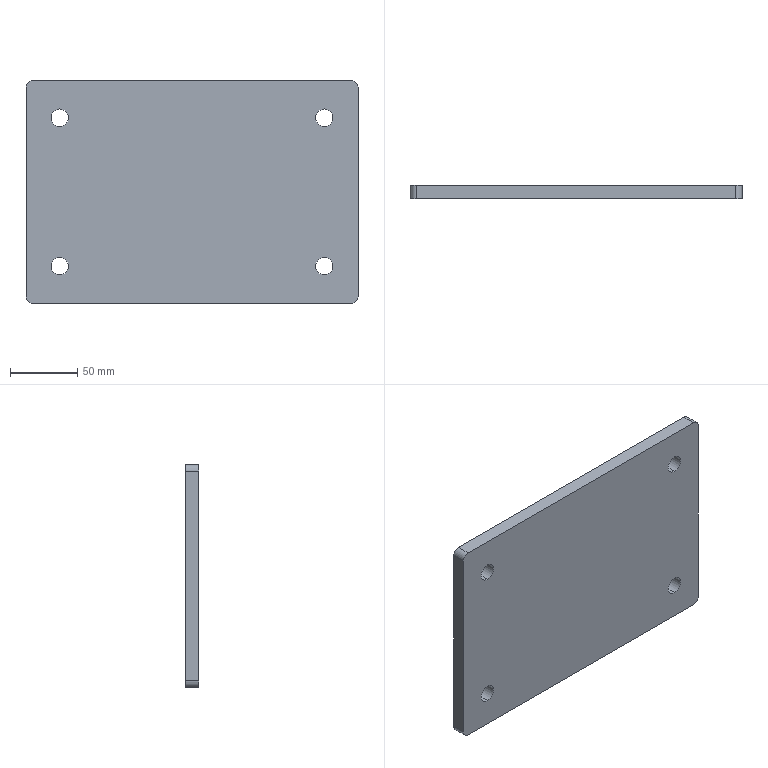Part | SolidWorks | features BaseBody 1 | 1 solid | 18 faces | box 246 x 10 x 165 mm | volume 400376 mm3 | cylinder 12 | plane 6 | commonest cylinder face diameters 13 x8 10 x4
STEP:
#1=CARTESIAN_POINT('',(-98.,0.,61.5));
#2=VERTEX_POINT('',#1);
#3=CARTESIAN_POINT('',(-98.,0.,48.5));
#4=VERTEX_POINT('',#3);
#5=CARTESIAN_POINT('',(-98.,0.,55.));
#6=DIRECTION('',(0.,-1.,0.));
#7=DIRECTION('',(0.,0.,1.));
#8=AXIS2_PLACEMENT_3D('',#5,#6,#7);
#9=CIRCLE('',#8,6.5);
#10=EDGE_CURVE('',#2,#4,#9,.T.);
#11=ORIENTED_EDGE('',*,*,#10,.T.);
#12=CARTESIAN_POINT('',(-98.,10.,48.5));
#13=VERTEX_POINT('',#12);
#14=CARTESIAN_POINT('',(-98.,-286.38,48.5));
#15=DIRECTION('',(0.,1.,0.));
#16=VECTOR('',#15,1000.);
#17=LINE('',#14,#16);
#18=EDGE_CURVE('',#4,#13,#17,.T.);
#19=ORIENTED_EDGE('',*,*,#18,.T.);
#20=CARTESIAN_POINT('',(-98.,10.,61.5));
#21=VERTEX_POINT('',#20);
#22=CARTESIAN_POINT('',(-98.,10.,55.));
#23=DIRECTION('',(0.,-1.,0.));
#24=DIRECTION('',(0.,0.,1.));
#25=AXIS2_PLACEMENT_3D('',#22,#23,#24);
#26=CIRCLE('',#25,6.5);
#27=EDGE_CURVE('',#21,#13,#26,.T.);
#28=ORIENTED_EDGE('',*,*,#27,.F.);
#29=CARTESIAN_POINT('',(-98.,-286.38,61.5));
#30=DIRECTION('',(0.,1.,0.));
#31=VECTOR('',#30,1000.);
#32=LINE('',#29,#31);
#33=EDGE_CURVE('',#2,#21,#32,.T.);
#34=ORIENTED_EDGE('',*,*,#33,.F.);
#35=EDGE_LOOP('',(#11,#19,#28,#34));
#36=FACE_OUTER_BOUND('',#35,.T.);
#37=CARTESIAN_POINT('',(-98.,-286.38,55.));
#38=DIRECTION('',(0.,1.,0.));
#39=DIRECTION('',(0.,0.,1.));
#40=AXIS2_PLACEMENT_3D('',#37,#38,#39);
#41=CYLINDRICAL_SURFACE('',#40,6.5);
#42=ADVANCED_FACE('',(#36),#41,.F.);
#43=CARTESIAN_POINT('',(-98.,0.,-48.5));
#44=VERTEX_POINT('',#43);
#45=CARTESIAN_POINT('',(-98.,0.,-61.5));
#46=VERTEX_POINT('',#45);
#47=CARTESIAN_POINT('',(-98.,0.,-55.));
#48=DIRECTION('',(0.,-1.,0.));
#49=DIRECTION('',(0.,0.,1.));
#50=AXIS2_PLACEMENT_3D('',#47,#48,#49);
#51=CIRCLE('',#50,6.5);
#52=EDGE_CURVE('',#44,#46,#51,.T.);
#53=ORIENTED_EDGE('',*,*,#52,.T.);
#54=CARTESIAN_POINT('',(-98.,10.,-61.5));
#55=VERTEX_POINT('',#54);
#56=CARTESIAN_POINT('',(-98.,-286.38,-61.5));
#57=DIRECTION('',(0.,1.,0.));
#58=VECTOR('',#57,1000.);
#59=LINE('',#56,#58);
#60=EDGE_CURVE('',#46,#55,#59,.T.);
#61=ORIENTED_EDGE('',*,*,#60,.T.);
#62=CARTESIAN_POINT('',(-98.,10.,-48.5));
#63=VERTEX_POINT('',#62);
#64=CARTESIAN_POINT('',(-98.,10.,-55.));
#65=DIRECTION('',(0.,-1.,0.));
#66=DIRECTION('',(0.,0.,1.));
#67=AXIS2_PLACEMENT_3D('',#64,#65,#66);
#68=CIRCLE('',#67,6.5);
#69=EDGE_CURVE('',#63,#55,#68,.T.);
#70=ORIENTED_EDGE('',*,*,#69,.F.);
#71=CARTESIAN_POINT('',(-98.,-286.38,-48.5));
#72=DIRECTION('',(0.,1.,0.));
#73=VECTOR('',#72,1000.);
#74=LINE('',#71,#73);
#75=EDGE_CURVE('',#44,#63,#74,.T.);
#76=ORIENTED_EDGE('',*,*,#75,.F.);
#77=EDGE_LOOP('',(#53,#61,#70,#76));
#78=FACE_OUTER_BOUND('',#77,.T.);
#79=CARTESIAN_POINT('',(-98.,-286.38,-55.));
#80=DIRECTION('',(0.,1.,0.));
#81=DIRECTION('',(0.,0.,1.));
#82=AXIS2_PLACEMENT_3D('',#79,#80,#81);
#83=CYLINDRICAL_SURFACE('',#82,6.5);
#84=ADVANCED_FACE('',(#78),#83,.F.);
#85=CARTESIAN_POINT('',(98.,0.,61.5));
#86=VERTEX_POINT('',#85);
#87=CARTESIAN_POINT('',(98.,0.,48.5));
#88=VERTEX_POINT('',#87);
#89=CARTESIAN_POINT('',(98.,0.,55.));
#90=DIRECTION('',(0.,-1.,0.));
#91=DIRECTION('',(0.,0.,1.));
#92=AXIS2_PLACEMENT_3D('',#89,#90,#91);
#93=CIRCLE('',#92,6.5);
#94=EDGE_CURVE('',#86,#88,#93,.T.);
#95=ORIENTED_EDGE('',*,*,#94,.T.);
#96=CARTESIAN_POINT('',(98.,10.,48.5));
#97=VERTEX_POINT('',#96);
#98=CARTESIAN_POINT('',(98.,-286.38,48.5));
#99=DIRECTION('',(0.,1.,0.));
#100=VECTOR('',#99,1000.);
#101=LINE('',#98,#100);
#102=EDGE_CURVE('',#88,#97,#101,.T.);
#103=ORIENTED_EDGE('',*,*,#102,.T.);
#104=CARTESIAN_POINT('',(98.,10.,61.5));
#105=VERTEX_POINT('',#104);
#106=CARTESIAN_POINT('',(98.,10.,55.));
#107=DIRECTION('',(0.,-1.,0.));
#108=DIRECTION('',(0.,0.,1.));
#109=AXIS2_PLACEMENT_3D('',#106,#107,#108);
#110=CIRCLE('',#109,6.5);
#111=EDGE_CURVE('',#105,#97,#110,.T.);
#112=ORIENTED_EDGE('',*,*,#111,.F.);
#113=CARTESIAN_POINT('',(98.,-286.38,61.5));
#114=DIRECTION('',(0.,1.,0.));
#115=VECTOR('',#114,1000.);
#116=LINE('',#113,#115);
#117=EDGE_CURVE('',#86,#105,#116,.T.);
#118=ORIENTED_EDGE('',*,*,#117,.F.);
#119=EDGE_LOOP('',(#95,#103,#112,#118));
#120=FACE_OUTER_BOUND('',#119,.T.);
#121=CARTESIAN_POINT('',(98.,-286.38,55.));
#122=DIRECTION('',(0.,1.,0.));
#123=DIRECTION('',(0.,0.,1.));
#124=AXIS2_PLACEMENT_3D('',#121,#122,#123);
#125=CYLINDRICAL_SURFACE('',#124,6.5);
#126=ADVANCED_FACE('',(#120),#125,.F.);
#127=CARTESIAN_POINT('',(98.,0.,-48.5));
#128=VERTEX_POINT('',#127);
#129=CARTESIAN_POINT('',(98.,0.,-61.5));
#130=VERTEX_POINT('',#129);
#131=CARTESIAN_POINT('',(98.,0.,-55.));
#132=DIRECTION('',(0.,-1.,0.));
#133=DIRECTION('',(0.,0.,1.));
#134=AXIS2_PLACEMENT_3D('',#131,#132,#133);
#135=CIRCLE('',#134,6.5);
#136=EDGE_CURVE('',#128,#130,#135,.T.);
#137=ORIENTED_EDGE('',*,*,#136,.T.);
#138=CARTESIAN_POINT('',(98.,10.,-61.5));
#139=VERTEX_POINT('',#138);
#140=CARTESIAN_POINT('',(98.,-286.38,-61.5));
#141=DIRECTION('',(0.,1.,0.));
#142=VECTOR('',#141,1000.);
#143=LINE('',#140,#142);
#144=EDGE_CURVE('',#130,#139,#143,.T.);
#145=ORIENTED_EDGE('',*,*,#144,.T.);
#146=CARTESIAN_POINT('',(98.,10.,-48.5));
#147=VERTEX_POINT('',#146);
#148=CARTESIAN_POINT('',(98.,10.,-55.));
#149=DIRECTION('',(0.,-1.,0.));
#150=DIRECTION('',(0.,0.,1.));
#151=AXIS2_PLACEMENT_3D('',#148,#149,#150);
#152=CIRCLE('',#151,6.5);
#153=EDGE_CURVE('',#147,#139,#152,.T.);
#154=ORIENTED_EDGE('',*,*,#153,.F.);
#155=CARTESIAN_POINT('',(98.,-286.38,-48.5));
#156=DIRECTION('',(0.,1.,0.));
#157=VECTOR('',#156,1000.);
#158=LINE('',#155,#157);
#159=EDGE_CURVE('',#128,#147,#158,.T.);
#160=ORIENTED_EDGE('',*,*,#159,.F.);
#161=EDGE_LOOP('',(#137,#145,#154,#160));
#162=FACE_OUTER_BOUND('',#161,.T.);
#163=CARTESIAN_POINT('',(98.,-286.38,-55.));
#164=DIRECTION('',(0.,1.,0.));
#165=DIRECTION('',(0.,0.,1.));
#166=AXIS2_PLACEMENT_3D('',#163,#164,#165);
#167=CYLINDRICAL_SURFACE('',#166,6.5);
#168=ADVANCED_FACE('',(#162),#167,.F.);
#169=ORIENTED_EDGE('',*,*,#10,.F.);
#170=CARTESIAN_POINT('',(-98.,0.,55.));
#171=DIRECTION('',(0.,-1.,0.));
#172=DIRECTION('',(0.,0.,1.));
#173=AXIS2_PLACEMENT_3D('',#170,#171,#172);
#174=CIRCLE('',#173,6.5);
#175=EDGE_CURVE('',#4,#2,#174,.T.);
#176=ORIENTED_EDGE('',*,*,#175,.F.);
#177=EDGE_LOOP('',(#169,#176));
#178=FACE_BOUND('',#177,.T.);
#179=ORIENTED_EDGE('',*,*,#52,.F.);
#180=CARTESIAN_POINT('',(-98.,0.,-55.));
#181=DIRECTION('',(0.,-1.,0.));
#182=DIRECTION('',(0.,0.,1.));
#183=AXIS2_PLACEMENT_3D('',#180,#181,#182);
#184=CIRCLE('',#183,6.5);
#185=EDGE_CURVE('',#46,#44,#184,.T.);
#186=ORIENTED_EDGE('',*,*,#185,.F.);
#187=EDGE_LOOP('',(#179,#186));
#188=FACE_BOUND('',#187,.T.);
#189=ORIENTED_EDGE('',*,*,#94,.F.);
#190=CARTESIAN_POINT('',(98.,0.,55.));
#191=DIRECTION('',(0.,-1.,0.));
#192=DIRECTION('',(0.,0.,1.));
#193=AXIS2_PLACEMENT_3D('',#190,#191,#192);
#194=CIRCLE('',#193,6.5);
#195=EDGE_CURVE('',#88,#86,#194,.T.);
#196=ORIENTED_EDGE('',*,*,#195,.F.);
#197=EDGE_LOOP('',(#189,#196));
#198=FACE_BOUND('',#197,.T.);
#199=ORIENTED_EDGE('',*,*,#136,.F.);
#200=CARTESIAN_POINT('',(98.,0.,-55.));
#201=DIRECTION('',(0.,-1.,0.));
#202=DIRECTION('',(0.,0.,1.));
#203=AXIS2_PLACEMENT_3D('',#200,#201,#202);
#204=CIRCLE('',#203,6.5);
#205=EDGE_CURVE('',#130,#128,#204,.T.);
#206=ORIENTED_EDGE('',*,*,#205,.F.);
#207=EDGE_LOOP('',(#199,#206));
#208=FACE_BOUND('',#207,.T.);
#209=CARTESIAN_POINT('',(118.,0.,-82.5));
#210=VERTEX_POINT('',#209);
#211=CARTESIAN_POINT('',(-118.,0.,-82.5));
#212=VERTEX_POINT('',#211);
#213=CARTESIAN_POINT('',(0.,0.,-82.5));
#214=DIRECTION('',(-1.,0.,0.));
#215=VECTOR('',#214,1000.);
#216=LINE('',#213,#215);
#217=EDGE_CURVE('',#210,#212,#216,.T.);
#218=ORIENTED_EDGE('',*,*,#217,.F.);
#219=CARTESIAN_POINT('',(123.,0.,-77.5));
#220=VERTEX_POINT('',#219);
#221=CARTESIAN_POINT('',(118.,0.,-77.5));
#222=DIRECTION('',(0.,1.,0.));
#223=DIRECTION('',(0.,0.,1.));
#224=AXIS2_PLACEMENT_3D('',#221,#222,#223);
#225=CIRCLE('',#224,5.);
#226=EDGE_CURVE('',#220,#210,#225,.T.);
#227=ORIENTED_EDGE('',*,*,#226,.F.);
#228=CARTESIAN_POINT('',(123.,0.,77.5));
#229=VERTEX_POINT('',#228);
#230=CARTESIAN_POINT('',(123.,0.,0.));
#231=DIRECTION('',(0.,0.,-1.));
#232=VECTOR('',#231,1000.);
#233=LINE('',#230,#232);
#234=EDGE_CURVE('',#229,#220,#233,.T.);
#235=ORIENTED_EDGE('',*,*,#234,.F.);
#236=CARTESIAN_POINT('',(118.,0.,82.5));
#237=VERTEX_POINT('',#236);
#238=CARTESIAN_POINT('',(118.,0.,77.5));
#239=DIRECTION('',(0.,1.,0.));
#240=DIRECTION('',(0.,0.,1.));
#241=AXIS2_PLACEMENT_3D('',#238,#239,#240);
#242=CIRCLE('',#241,5.);
#243=EDGE_CURVE('',#237,#229,#242,.T.);
#244=ORIENTED_EDGE('',*,*,#243,.F.);
#245=CARTESIAN_POINT('',(-118.,0.,82.5));
#246=VERTEX_POINT('',#245);
#247=CARTESIAN_POINT('',(0.,0.,82.5));
#248=DIRECTION('',(1.,0.,0.));
#249=VECTOR('',#248,1000.);
#250=LINE('',#247,#249);
#251=EDGE_CURVE('',#246,#237,#250,.T.);
#252=ORIENTED_EDGE('',*,*,#251,.F.);
#253=CARTESIAN_POINT('',(-123.,0.,77.5));
#254=VERTEX_POINT('',#253);
#255=CARTESIAN_POINT('',(-118.,0.,77.5));
#256=DIRECTION('',(0.,1.,0.));
#257=DIRECTION('',(0.,0.,1.));
#258=AXIS2_PLACEMENT_3D('',#255,#256,#257);
#259=CIRCLE('',#258,5.);
#260=EDGE_CURVE('',#254,#246,#259,.T.);
#261=ORIENTED_EDGE('',*,*,#260,.F.);
#262=CARTESIAN_POINT('',(-123.,0.,-77.5));
#263=VERTEX_POINT('',#262);
#264=CARTESIAN_POINT('',(-123.,0.,0.));
#265=DIRECTION('',(0.,0.,1.));
#266=VECTOR('',#265,1000.);
#267=LINE('',#264,#266);
#268=EDGE_CURVE('',#263,#254,#267,.T.);
#269=ORIENTED_EDGE('',*,*,#268,.F.);
#270=CARTESIAN_POINT('',(-118.,0.,-77.5));
#271=DIRECTION('',(0.,1.,0.));
#272=DIRECTION('',(0.,0.,1.));
#273=AXIS2_PLACEMENT_3D('',#270,#271,#272);
#274=CIRCLE('',#273,5.);
#275=EDGE_CURVE('',#212,#263,#274,.T.);
#276=ORIENTED_EDGE('',*,*,#275,.F.);
#277=EDGE_LOOP('',(#218,#227,#235,#244,#252,#261,#269,#276));
#278=FACE_OUTER_BOUND('',#277,.T.);
#279=CARTESIAN_POINT('',(0.,0.,0.));
#280=DIRECTION('',(0.,1.,0.));
#281=DIRECTION('',(0.,0.,1.));
#282=AXIS2_PLACEMENT_3D('',#279,#280,#281);
#283=PLANE('',#282);
#284=ADVANCED_FACE('',(#178,#188,#198,#208,#278),#283,.F.);
#285=ORIENTED_EDGE('',*,*,#18,.F.);
#286=ORIENTED_EDGE('',*,*,#175,.T.);
#287=ORIENTED_EDGE('',*,*,#33,.T.);
#288=CARTESIAN_POINT('',(-98.,10.,55.));
#289=DIRECTION('',(0.,-1.,0.));
#290=DIRECTION('',(0.,0.,1.));
#291=AXIS2_PLACEMENT_3D('',#288,#289,#290);
#292=CIRCLE('',#291,6.5);
#293=EDGE_CURVE('',#13,#21,#292,.T.);
#294=ORIENTED_EDGE('',*,*,#293,.F.);
#295=EDGE_LOOP('',(#285,#286,#287,#294));
#296=FACE_OUTER_BOUND('',#295,.T.);
#297=CARTESIAN_POINT('',(-98.,-286.38,55.));
#298=DIRECTION('',(0.,1.,0.));
#299=DIRECTION('',(0.,0.,1.));
#300=AXIS2_PLACEMENT_3D('',#297,#298,#299);
#301=CYLINDRICAL_SURFACE('',#300,6.5);
#302=ADVANCED_FACE('',(#296),#301,.F.);
#303=ORIENTED_EDGE('',*,*,#60,.F.);
#304=ORIENTED_EDGE('',*,*,#185,.T.);
#305=ORIENTED_EDGE('',*,*,#75,.T.);
#306=CARTESIAN_POINT('',(-98.,10.,-55.));
#307=DIRECTION('',(0.,-1.,0.));
#308=DIRECTION('',(0.,0.,1.));
#309=AXIS2_PLACEMENT_3D('',#306,#307,#308);
#310=CIRCLE('',#309,6.5);
#311=EDGE_CURVE('',#55,#63,#310,.T.);
#312=ORIENTED_EDGE('',*,*,#311,.F.);
#313=EDGE_LOOP('',(#303,#304,#305,#312));
#314=FACE_OUTER_BOUND('',#313,.T.);
#315=CARTESIAN_POINT('',(-98.,-286.38,-55.));
#316=DIRECTION('',(0.,1.,0.));
#317=DIRECTION('',(0.,0.,1.));
#318=AXIS2_PLACEMENT_3D('',#315,#316,#317);
#319=CYLINDRICAL_SURFACE('',#318,6.5);
#320=ADVANCED_FACE('',(#314),#319,.F.);
#321=ORIENTED_EDGE('',*,*,#102,.F.);
#322=ORIENTED_EDGE('',*,*,#195,.T.);
#323=ORIENTED_EDGE('',*,*,#117,.T.);
#324=CARTESIAN_POINT('',(98.,10.,55.));
#325=DIRECTION('',(0.,-1.,0.));
#326=DIRECTION('',(0.,0.,1.));
#327=AXIS2_PLACEMENT_3D('',#324,#325,#326);
#328=CIRCLE('',#327,6.5);
#329=EDGE_CURVE('',#97,#105,#328,.T.);
#330=ORIENTED_EDGE('',*,*,#329,.F.);
#331=EDGE_LOOP('',(#321,#322,#323,#330));
#332=FACE_OUTER_BOUND('',#331,.T.);
#333=CARTESIAN_POINT('',(98.,-286.38,55.));
#334=DIRECTION('',(0.,1.,0.));
#335=DIRECTION('',(0.,0.,1.));
#336=AXIS2_PLACEMENT_3D('',#333,#334,#335);
#337=CYLINDRICAL_SURFACE('',#336,6.5);
#338=ADVANCED_FACE('',(#332),#337,.F.);
#339=ORIENTED_EDGE('',*,*,#144,.F.);
#340=ORIENTED_EDGE('',*,*,#205,.T.);
#341=ORIENTED_EDGE('',*,*,#159,.T.);
#342=CARTESIAN_POINT('',(98.,10.,-55.));
#343=DIRECTION('',(0.,-1.,0.));
#344=DIRECTION('',(0.,0.,1.));
#345=AXIS2_PLACEMENT_3D('',#342,#343,#344);
#346=CIRCLE('',#345,6.5);
#347=EDGE_CURVE('',#139,#147,#346,.T.);
#348=ORIENTED_EDGE('',*,*,#347,.F.);
#349=EDGE_LOOP('',(#339,#340,#341,#348));
#350=FACE_OUTER_BOUND('',#349,.T.);
#351=CARTESIAN_POINT('',(98.,-286.38,-55.));
#352=DIRECTION('',(0.,1.,0.));
#353=DIRECTION('',(0.,0.,1.));
#354=AXIS2_PLACEMENT_3D('',#351,#352,#353);
#355=CYLINDRICAL_SURFACE('',#354,6.5);
#356=ADVANCED_FACE('',(#350),#355,.F.);
#357=ORIENTED_EDGE('',*,*,#275,.T.);
#358=CARTESIAN_POINT('',(-123.,10.,-77.5));
#359=VERTEX_POINT('',#358);
#360=CARTESIAN_POINT('',(-123.,0.,-77.5));
#361=DIRECTION('',(0.,1.,0.));
#362=VECTOR('',#361,1000.);
#363=LINE('',#360,#362);
#364=EDGE_CURVE('',#263,#359,#363,.T.);
#365=ORIENTED_EDGE('',*,*,#364,.T.);
#366=CARTESIAN_POINT('',(-118.,10.,-82.5));
#367=VERTEX_POINT('',#366);
#368=CARTESIAN_POINT('',(-118.,10.,-77.5));
#369=DIRECTION('',(0.,-1.,0.));
#370=DIRECTION('',(0.,0.,1.));
#371=AXIS2_PLACEMENT_3D('',#368,#369,#370);
#372=CIRCLE('',#371,5.);
#373=EDGE_CURVE('',#359,#367,#372,.T.);
#374=ORIENTED_EDGE('',*,*,#373,.T.);
#375=CARTESIAN_POINT('',(-118.,0.,-82.5));
#376=DIRECTION('',(0.,-1.,0.));
#377=VECTOR('',#376,1000.);
#378=LINE('',#375,#377);
#379=EDGE_CURVE('',#367,#212,#378,.T.);
#380=ORIENTED_EDGE('',*,*,#379,.T.);
#381=EDGE_LOOP('',(#357,#365,#374,#380));
#382=FACE_OUTER_BOUND('',#381,.T.);
#383=CARTESIAN_POINT('',(-118.,0.,-77.5));
#384=DIRECTION('',(0.,1.,0.));
#385=DIRECTION('',(0.,0.,1.));
#386=AXIS2_PLACEMENT_3D('',#383,#384,#385);
#387=CYLINDRICAL_SURFACE('',#386,5.);
#388=ADVANCED_FACE('',(#382),#387,.T.);
#389=CARTESIAN_POINT('',(118.,10.,-82.5));
#390=VERTEX_POINT('',#389);
#391=CARTESIAN_POINT('',(118.,0.,-82.5));
#392=DIRECTION('',(0.,-1.,0.));
#393=VECTOR('',#392,1000.);
#394=LINE('',#391,#393);
#395=EDGE_CURVE('',#390,#210,#394,.T.);
#396=ORIENTED_EDGE('',*,*,#395,.T.);
#397=ORIENTED_EDGE('',*,*,#217,.T.);
#398=ORIENTED_EDGE('',*,*,#379,.F.);
#399=CARTESIAN_POINT('',(123.,10.,-82.5));
#400=DIRECTION('',(1.,0.,0.));
#401=VECTOR('',#400,1000.);
#402=LINE('',#399,#401);
#403=EDGE_CURVE('',#367,#390,#402,.T.);
#404=ORIENTED_EDGE('',*,*,#403,.T.);
#405=EDGE_LOOP('',(#396,#397,#398,#404));
#406=FACE_OUTER_BOUND('',#405,.T.);
#407=CARTESIAN_POINT('',(123.,0.,-82.5));
#408=DIRECTION('',(0.,0.,-1.));
#409=DIRECTION('',(-1.,0.,0.));
#410=AXIS2_PLACEMENT_3D('',#407,#408,#409);
#411=PLANE('',#410);
#412=ADVANCED_FACE('',(#406),#411,.T.);
#413=ORIENTED_EDGE('',*,*,#226,.T.);
#414=ORIENTED_EDGE('',*,*,#395,.F.);
#415=CARTESIAN_POINT('',(123.,10.,-77.5));
#416=VERTEX_POINT('',#415);
#417=CARTESIAN_POINT('',(118.,10.,-77.5));
#418=DIRECTION('',(0.,-1.,0.));
#419=DIRECTION('',(0.,0.,1.));
#420=AXIS2_PLACEMENT_3D('',#417,#418,#419);
#421=CIRCLE('',#420,5.);
#422=EDGE_CURVE('',#390,#416,#421,.T.);
#423=ORIENTED_EDGE('',*,*,#422,.T.);
#424=CARTESIAN_POINT('',(123.,0.,-77.5));
#425=DIRECTION('',(0.,-1.,0.));
#426=VECTOR('',#425,1000.);
#427=LINE('',#424,#426);
#428=EDGE_CURVE('',#416,#220,#427,.T.);
#429=ORIENTED_EDGE('',*,*,#428,.T.);
#430=EDGE_LOOP('',(#413,#414,#423,#429));
#431=FACE_OUTER_BOUND('',#430,.T.);
#432=CARTESIAN_POINT('',(118.,0.,-77.5));
#433=DIRECTION('',(0.,1.,0.));
#434=DIRECTION('',(0.,0.,1.));
#435=AXIS2_PLACEMENT_3D('',#432,#433,#434);
#436=CYLINDRICAL_SURFACE('',#435,5.);
#437=ADVANCED_FACE('',(#431),#436,.T.);
#438=CARTESIAN_POINT('',(123.,10.,77.5));
#439=VERTEX_POINT('',#438);
#440=CARTESIAN_POINT('',(123.,0.,77.5));
#441=DIRECTION('',(0.,-1.,0.));
#442=VECTOR('',#441,1000.);
#443=LINE('',#440,#442);
#444=EDGE_CURVE('',#439,#229,#443,.T.);
#445=ORIENTED_EDGE('',*,*,#444,.T.);
#446=ORIENTED_EDGE('',*,*,#234,.T.);
#447=ORIENTED_EDGE('',*,*,#428,.F.);
#448=CARTESIAN_POINT('',(123.,10.,82.5));
#449=DIRECTION('',(0.,0.,1.));
#450=VECTOR('',#449,1000.);
#451=LINE('',#448,#450);
#452=EDGE_CURVE('',#416,#439,#451,.T.);
#453=ORIENTED_EDGE('',*,*,#452,.T.);
#454=EDGE_LOOP('',(#445,#446,#447,#453));
#455=FACE_OUTER_BOUND('',#454,.T.);
#456=CARTESIAN_POINT('',(123.,0.,82.5));
#457=DIRECTION('',(1.,0.,0.));
#458=DIRECTION('',(0.,0.,-1.));
#459=AXIS2_PLACEMENT_3D('',#456,#457,#458);
#460=PLANE('',#459);
#461=ADVANCED_FACE('',(#455),#460,.T.);
#462=ORIENTED_EDGE('',*,*,#243,.T.);
#463=ORIENTED_EDGE('',*,*,#444,.F.);
#464=CARTESIAN_POINT('',(118.,10.,82.5));
#465=VERTEX_POINT('',#464);
#466=CARTESIAN_POINT('',(118.,10.,77.5));
#467=DIRECTION('',(0.,-1.,0.));
#468=DIRECTION('',(0.,0.,1.));
#469=AXIS2_PLACEMENT_3D('',#466,#467,#468);
#470=CIRCLE('',#469,5.);
#471=EDGE_CURVE('',#439,#465,#470,.T.);
#472=ORIENTED_EDGE('',*,*,#471,.T.);
#473=CARTESIAN_POINT('',(118.,0.,82.5));
#474=DIRECTION('',(0.,-1.,0.));
#475=VECTOR('',#474,1000.);
#476=LINE('',#473,#475);
#477=EDGE_CURVE('',#465,#237,#476,.T.);
#478=ORIENTED_EDGE('',*,*,#477,.T.);
#479=EDGE_LOOP('',(#462,#463,#472,#478));
#480=FACE_OUTER_BOUND('',#479,.T.);
#481=CARTESIAN_POINT('',(118.,0.,77.5));
#482=DIRECTION('',(0.,1.,0.));
#483=DIRECTION('',(0.,0.,1.));
#484=AXIS2_PLACEMENT_3D('',#481,#482,#483);
#485=CYLINDRICAL_SURFACE('',#484,5.);
#486=ADVANCED_FACE('',(#480),#485,.T.);
#487=CARTESIAN_POINT('',(-118.,10.,82.5));
#488=VERTEX_POINT('',#487);
#489=CARTESIAN_POINT('',(-118.,0.,82.5));
#490=DIRECTION('',(0.,-1.,0.));
#491=VECTOR('',#490,1000.);
#492=LINE('',#489,#491);
#493=EDGE_CURVE('',#488,#246,#492,.T.);
#494=ORIENTED_EDGE('',*,*,#493,.T.);
#495=ORIENTED_EDGE('',*,*,#251,.T.);
#496=ORIENTED_EDGE('',*,*,#477,.F.);
#497=CARTESIAN_POINT('',(-123.,10.,82.5));
#498=DIRECTION('',(-1.,0.,0.));
#499=VECTOR('',#498,1000.);
#500=LINE('',#497,#499);
#501=EDGE_CURVE('',#465,#488,#500,.T.);
#502=ORIENTED_EDGE('',*,*,#501,.T.);
#503=EDGE_LOOP('',(#494,#495,#496,#502));
#504=FACE_OUTER_BOUND('',#503,.T.);
#505=CARTESIAN_POINT('',(-123.,0.,82.5));
#506=DIRECTION('',(0.,0.,1.));
#507=DIRECTION('',(1.,0.,0.));
#508=AXIS2_PLACEMENT_3D('',#505,#506,#507);
#509=PLANE('',#508);
#510=ADVANCED_FACE('',(#504),#509,.T.);
#511=ORIENTED_EDGE('',*,*,#260,.T.);
#512=ORIENTED_EDGE('',*,*,#493,.F.);
#513=CARTESIAN_POINT('',(-123.,10.,77.5));
#514=VERTEX_POINT('',#513);
#515=CARTESIAN_POINT('',(-118.,10.,77.5));
#516=DIRECTION('',(0.,-1.,0.));
#517=DIRECTION('',(0.,0.,1.));
#518=AXIS2_PLACEMENT_3D('',#515,#516,#517);
#519=CIRCLE('',#518,5.);
#520=EDGE_CURVE('',#488,#514,#519,.T.);
#521=ORIENTED_EDGE('',*,*,#520,.T.);
#522=CARTESIAN_POINT('',(-123.,0.,77.5));
#523=DIRECTION('',(0.,-1.,0.));
#524=VECTOR('',#523,1000.);
#525=LINE('',#522,#524);
#526=EDGE_CURVE('',#514,#254,#525,.T.);
#527=ORIENTED_EDGE('',*,*,#526,.T.);
#528=EDGE_LOOP('',(#511,#512,#521,#527));
#529=FACE_OUTER_BOUND('',#528,.T.);
#530=CARTESIAN_POINT('',(-118.,0.,77.5));
#531=DIRECTION('',(0.,1.,0.));
#532=DIRECTION('',(0.,0.,1.));
#533=AXIS2_PLACEMENT_3D('',#530,#531,#532);
#534=CYLINDRICAL_SURFACE('',#533,5.);
#535=ADVANCED_FACE('',(#529),#534,.T.);
#536=ORIENTED_EDGE('',*,*,#526,.F.);
#537=CARTESIAN_POINT('',(-123.,10.,-82.5));
#538=DIRECTION('',(0.,0.,-1.));
#539=VECTOR('',#538,1000.);
#540=LINE('',#537,#539);
#541=EDGE_CURVE('',#514,#359,#540,.T.);
#542=ORIENTED_EDGE('',*,*,#541,.T.);
#543=ORIENTED_EDGE('',*,*,#364,.F.);
#544=ORIENTED_EDGE('',*,*,#268,.T.);
#545=EDGE_LOOP('',(#536,#542,#543,#544));
#546=FACE_OUTER_BOUND('',#545,.T.);
#547=CARTESIAN_POINT('',(-123.,0.,-82.5));
#548=DIRECTION('',(-1.,0.,0.));
#549=DIRECTION('',(0.,0.,1.));
#550=AXIS2_PLACEMENT_3D('',#547,#548,#549);
#551=PLANE('',#550);
#552=ADVANCED_FACE('',(#546),#551,.T.);
#553=ORIENTED_EDGE('',*,*,#27,.T.);
#554=ORIENTED_EDGE('',*,*,#293,.T.);
#555=EDGE_LOOP('',(#553,#554));
#556=FACE_BOUND('',#555,.T.);
#557=ORIENTED_EDGE('',*,*,#69,.T.);
#558=ORIENTED_EDGE('',*,*,#311,.T.);
#559=EDGE_LOOP('',(#557,#558));
#560=FACE_BOUND('',#559,.T.);
#561=ORIENTED_EDGE('',*,*,#111,.T.);
#562=ORIENTED_EDGE('',*,*,#329,.T.);
#563=EDGE_LOOP('',(#561,#562));
#564=FACE_BOUND('',#563,.T.);
#565=ORIENTED_EDGE('',*,*,#153,.T.);
#566=ORIENTED_EDGE('',*,*,#347,.T.);
#567=EDGE_LOOP('',(#565,#566));
#568=FACE_BOUND('',#567,.T.);
#569=ORIENTED_EDGE('',*,*,#422,.F.);
#570=ORIENTED_EDGE('',*,*,#403,.F.);
#571=ORIENTED_EDGE('',*,*,#373,.F.);
#572=ORIENTED_EDGE('',*,*,#541,.F.);
#573=ORIENTED_EDGE('',*,*,#520,.F.);
#574=ORIENTED_EDGE('',*,*,#501,.F.);
#575=ORIENTED_EDGE('',*,*,#471,.F.);
#576=ORIENTED_EDGE('',*,*,#452,.F.);
#577=EDGE_LOOP('',(#569,#570,#571,#572,#573,#574,#575,#576));
#578=FACE_OUTER_BOUND('',#577,.T.);
#579=CARTESIAN_POINT('',(0.,10.,0.));
#580=DIRECTION('',(0.,1.,0.));
#581=DIRECTION('',(0.,0.,1.));
#582=AXIS2_PLACEMENT_3D('',#579,#580,#581);
#583=PLANE('',#582);
#584=ADVANCED_FACE('',(#556,#560,#564,#568,#578),#583,.T.);
#585=CLOSED_SHELL('',(#42,#84,#126,#168,#284,#302,#320,#338,#356,#388,#412,#437,#461,#486,#510,#535,#552,#584));
#586=MANIFOLD_SOLID_BREP('',#585);
#587=CARTESIAN_POINT('',(0.,0.,0.));
#588=DIRECTION('',(0.,0.,1.));
#589=DIRECTION('',(1.,0.,0.));
#590=AXIS2_PLACEMENT_3D('',#587,#588,#589);
#591=(LENGTH_UNIT()NAMED_UNIT(*)SI_UNIT(.MILLI.,.METRE.));
#592=UNCERTAINTY_MEASURE_WITH_UNIT(LENGTH_MEASURE(0.00001),#591,'','');
#593=(NAMED_UNIT(*)PLANE_ANGLE_UNIT()SI_UNIT($,.RADIAN.));
#594=(NAMED_UNIT(*)SI_UNIT($,.STERADIAN.)SOLID_ANGLE_UNIT());
#595=(GEOMETRIC_REPRESENTATION_CONTEXT(3)GLOBAL_UNCERTAINTY_ASSIGNED_CONTEXT((#592))GLOBAL_UNIT_ASSIGNED_CONTEXT((#591,#593,#594))REPRESENTATION_CONTEXT('',''));
#596=ADVANCED_BREP_SHAPE_REPRESENTATION('',(#586,#590),#595);